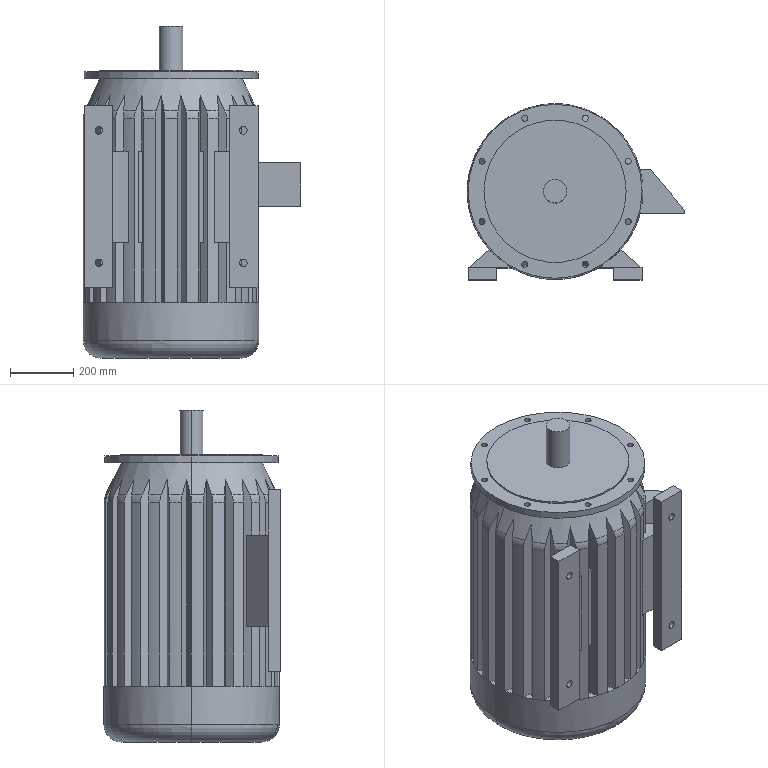Part | SolidWorks | features Boss 7, Cut 3, CirPattern 2, Chamfer 1, Extrusion 1, Fillet 1 | 1 solid | 191 faces | box 687.6 x 557.6 x 1050 mm | volume 215841244 mm3 | plane 99 | cylinder 62 | torus 28 | cone 2 | commonest cylinder face diameters 555 x30 19 x16 24 x8 75 x2 450 x2 550 x2